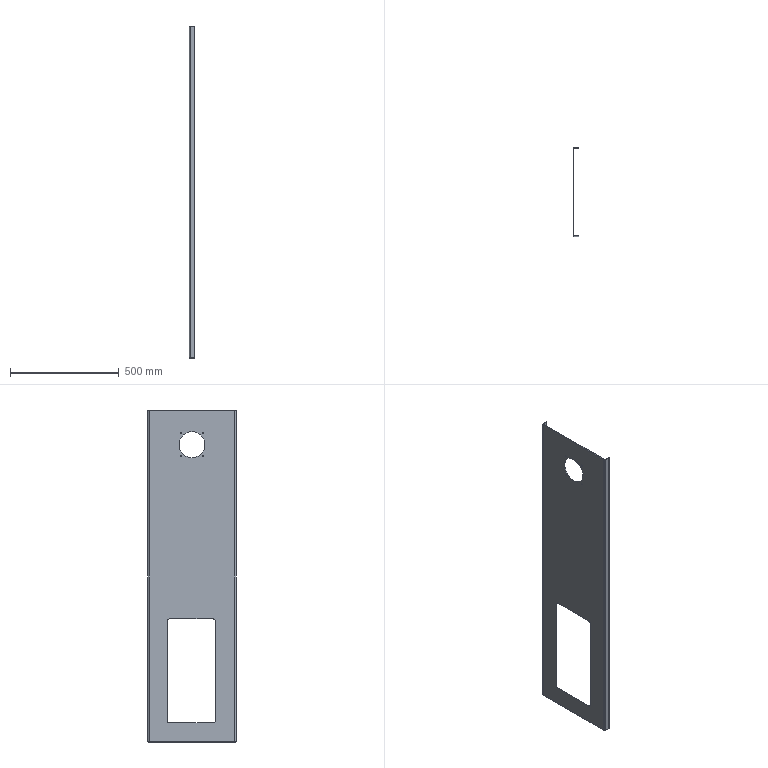Part | STEP file | ASND-0110-E63-HLTP01标准Lower机架-08 | 1 solid | 44 faces | box 26.5 x 408 x 1530 mm | volume 863375 mm3 | cylinder 28 | plane 12 | torus 4 | commonest cylinder face diameters 5.5 x8 20 x8 6 x6 10 x2 13 x2 120 x2